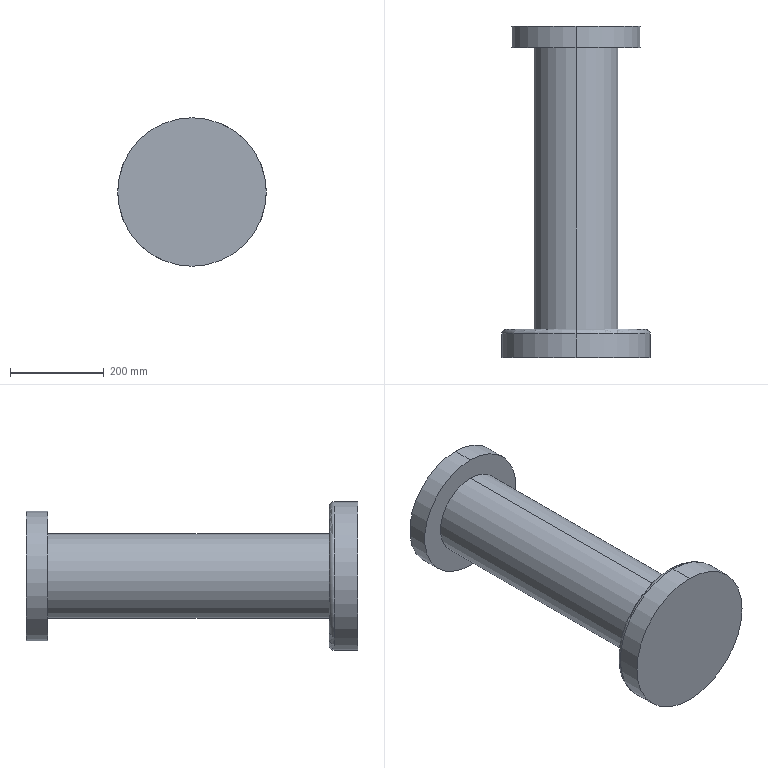Part | SolidWorks | features ICE 2, Extrusion 1, Fillet 1 | 1 solid | 12 faces | box 316.364 x 705 x 316.364 mm | volume 22636383 mm3 | cylinder 6 | plane 4 | torus 2 | commonest cylinder face diameters 180 x2 275 x2 316.364 x2
STEP:
#1=CARTESIAN_POINT('',(0.,-600.,148.182));
#2=VERTEX_POINT('',#1);
#3=CARTESIAN_POINT('',(0.,-600.,-148.182));
#4=VERTEX_POINT('',#3);
#5=CARTESIAN_POINT('',(0.,-600.,0.));
#6=DIRECTION('',(0.,1.,0.));
#7=DIRECTION('',(0.,0.,-1.));
#8=AXIS2_PLACEMENT_3D('',#5,#6,#7);
#9=CIRCLE('',#8,148.182);
#10=EDGE_CURVE('',#2,#4,#9,.T.);
#11=ORIENTED_EDGE('',*,*,#10,.F.);
#12=CARTESIAN_POINT('',(0.,-610.,158.182));
#13=VERTEX_POINT('',#12);
#14=CARTESIAN_POINT('',(0.,-610.,148.182));
#15=DIRECTION('',(1.,0.,0.));
#16=DIRECTION('',(0.,0.,-1.));
#17=AXIS2_PLACEMENT_3D('',#14,#15,#16);
#18=CIRCLE('',#17,10.);
#19=EDGE_CURVE('',#2,#13,#18,.T.);
#20=ORIENTED_EDGE('',*,*,#19,.T.);
#21=CARTESIAN_POINT('',(0.,-610.,-158.182));
#22=VERTEX_POINT('',#21);
#23=CARTESIAN_POINT('',(0.,-610.,0.));
#24=DIRECTION('',(0.,-1.,0.));
#25=DIRECTION('',(0.,0.,-1.));
#26=AXIS2_PLACEMENT_3D('',#23,#24,#25);
#27=CIRCLE('',#26,158.182);
#28=EDGE_CURVE('',#22,#13,#27,.T.);
#29=ORIENTED_EDGE('',*,*,#28,.F.);
#30=CARTESIAN_POINT('',(0.,-610.,-148.182));
#31=DIRECTION('',(-1.,0.,0.));
#32=DIRECTION('',(0.,0.,1.));
#33=AXIS2_PLACEMENT_3D('',#30,#31,#32);
#34=CIRCLE('',#33,10.);
#35=EDGE_CURVE('',#4,#22,#34,.T.);
#36=ORIENTED_EDGE('',*,*,#35,.F.);
#37=EDGE_LOOP('',(#11,#20,#29,#36));
#38=FACE_OUTER_BOUND('',#37,.T.);
#39=CARTESIAN_POINT('',(0.,-610.,0.));
#40=DIRECTION('',(0.,-1.,0.));
#41=DIRECTION('',(0.,0.,-1.));
#42=AXIS2_PLACEMENT_3D('',#39,#40,#41);
#43=TOROIDAL_SURFACE('',#42,148.182,10.);
#44=ADVANCED_FACE('',(#38),#43,.T.);
#45=CARTESIAN_POINT('',(0.,-660.,-158.182));
#46=VERTEX_POINT('',#45);
#47=CARTESIAN_POINT('',(0.,-660.,158.182));
#48=VERTEX_POINT('',#47);
#49=CARTESIAN_POINT('',(0.,-660.,0.));
#50=DIRECTION('',(0.,-1.,0.));
#51=DIRECTION('',(0.,0.,-1.));
#52=AXIS2_PLACEMENT_3D('',#49,#50,#51);
#53=CIRCLE('',#52,158.182);
#54=EDGE_CURVE('',#46,#48,#53,.T.);
#55=ORIENTED_EDGE('',*,*,#54,.F.);
#56=CARTESIAN_POINT('',(0.,-660.,-158.182));
#57=DIRECTION('',(0.,1.,0.));
#58=VECTOR('',#57,1000.);
#59=LINE('',#56,#58);
#60=EDGE_CURVE('',#46,#22,#59,.T.);
#61=ORIENTED_EDGE('',*,*,#60,.T.);
#62=ORIENTED_EDGE('',*,*,#28,.T.);
#63=CARTESIAN_POINT('',(0.,-660.,158.182));
#64=DIRECTION('',(0.,1.,0.));
#65=VECTOR('',#64,1000.);
#66=LINE('',#63,#65);
#67=EDGE_CURVE('',#48,#13,#66,.T.);
#68=ORIENTED_EDGE('',*,*,#67,.F.);
#69=EDGE_LOOP('',(#55,#61,#62,#68));
#70=FACE_OUTER_BOUND('',#69,.T.);
#71=CARTESIAN_POINT('',(0.,-660.,0.));
#72=DIRECTION('',(0.,1.,0.));
#73=DIRECTION('',(0.,0.,1.));
#74=AXIS2_PLACEMENT_3D('',#71,#72,#73);
#75=CYLINDRICAL_SURFACE('',#74,158.182);
#76=ADVANCED_FACE('',(#70),#75,.T.);
#77=CARTESIAN_POINT('',(0.,-600.,-90.));
#78=VERTEX_POINT('',#77);
#79=CARTESIAN_POINT('',(0.,-600.,90.));
#80=VERTEX_POINT('',#79);
#81=CARTESIAN_POINT('',(0.,-600.,0.));
#82=DIRECTION('',(0.,-1.,0.));
#83=DIRECTION('',(0.,0.,-1.));
#84=AXIS2_PLACEMENT_3D('',#81,#82,#83);
#85=CIRCLE('',#84,90.);
#86=EDGE_CURVE('',#78,#80,#85,.T.);
#87=ORIENTED_EDGE('',*,*,#86,.F.);
#88=CARTESIAN_POINT('',(0.,0.,-90.));
#89=VERTEX_POINT('',#88);
#90=CARTESIAN_POINT('',(0.,-600.,-90.));
#91=DIRECTION('',(0.,1.,0.));
#92=VECTOR('',#91,1000.);
#93=LINE('',#90,#92);
#94=EDGE_CURVE('',#78,#89,#93,.T.);
#95=ORIENTED_EDGE('',*,*,#94,.T.);
#96=CARTESIAN_POINT('',(0.,0.,90.));
#97=VERTEX_POINT('',#96);
#98=CARTESIAN_POINT('',(0.,0.,0.));
#99=DIRECTION('',(0.,-1.,0.));
#100=DIRECTION('',(0.,0.,1.));
#101=AXIS2_PLACEMENT_3D('',#98,#99,#100);
#102=CIRCLE('',#101,90.);
#103=EDGE_CURVE('',#89,#97,#102,.T.);
#104=ORIENTED_EDGE('',*,*,#103,.T.);
#105=CARTESIAN_POINT('',(0.,-600.,90.));
#106=DIRECTION('',(0.,1.,0.));
#107=VECTOR('',#106,1000.);
#108=LINE('',#105,#107);
#109=EDGE_CURVE('',#80,#97,#108,.T.);
#110=ORIENTED_EDGE('',*,*,#109,.F.);
#111=EDGE_LOOP('',(#87,#95,#104,#110));
#112=FACE_OUTER_BOUND('',#111,.T.);
#113=CARTESIAN_POINT('',(0.,-600.,0.));
#114=DIRECTION('',(0.,1.,0.));
#115=DIRECTION('',(0.,0.,1.));
#116=AXIS2_PLACEMENT_3D('',#113,#114,#115);
#117=CYLINDRICAL_SURFACE('',#116,90.);
#118=ADVANCED_FACE('',(#112),#117,.T.);
#119=CARTESIAN_POINT('',(0.,45.,137.5));
#120=VERTEX_POINT('',#119);
#121=CARTESIAN_POINT('',(0.,45.,-137.5));
#122=VERTEX_POINT('',#121);
#123=CARTESIAN_POINT('',(0.,45.,0.));
#124=DIRECTION('',(0.,1.,0.));
#125=DIRECTION('',(0.,0.,1.));
#126=AXIS2_PLACEMENT_3D('',#123,#124,#125);
#127=CIRCLE('',#126,137.5);
#128=EDGE_CURVE('',#120,#122,#127,.T.);
#129=ORIENTED_EDGE('',*,*,#128,.F.);
#130=CARTESIAN_POINT('',(0.,0.,137.5));
#131=VERTEX_POINT('',#130);
#132=CARTESIAN_POINT('',(0.,45.,137.5));
#133=DIRECTION('',(0.,-1.,0.));
#134=VECTOR('',#133,1000.);
#135=LINE('',#132,#134);
#136=EDGE_CURVE('',#120,#131,#135,.T.);
#137=ORIENTED_EDGE('',*,*,#136,.T.);
#138=CARTESIAN_POINT('',(0.,0.,-137.5));
#139=VERTEX_POINT('',#138);
#140=CARTESIAN_POINT('',(0.,0.,0.));
#141=DIRECTION('',(0.,1.,0.));
#142=DIRECTION('',(0.,0.,1.));
#143=AXIS2_PLACEMENT_3D('',#140,#141,#142);
#144=CIRCLE('',#143,137.5);
#145=EDGE_CURVE('',#131,#139,#144,.T.);
#146=ORIENTED_EDGE('',*,*,#145,.T.);
#147=CARTESIAN_POINT('',(0.,45.,-137.5));
#148=DIRECTION('',(0.,-1.,0.));
#149=VECTOR('',#148,1000.);
#150=LINE('',#147,#149);
#151=EDGE_CURVE('',#122,#139,#150,.T.);
#152=ORIENTED_EDGE('',*,*,#151,.F.);
#153=EDGE_LOOP('',(#129,#137,#146,#152));
#154=FACE_OUTER_BOUND('',#153,.T.);
#155=CARTESIAN_POINT('',(0.,45.,0.));
#156=DIRECTION('',(0.,-1.,0.));
#157=DIRECTION('',(0.,0.,-1.));
#158=AXIS2_PLACEMENT_3D('',#155,#156,#157);
#159=CYLINDRICAL_SURFACE('',#158,137.5);
#160=ADVANCED_FACE('',(#154),#159,.T.);
#161=ORIENTED_EDGE('',*,*,#136,.F.);
#162=CARTESIAN_POINT('',(0.,45.,0.));
#163=DIRECTION('',(0.,1.,0.));
#164=DIRECTION('',(0.,0.,1.));
#165=AXIS2_PLACEMENT_3D('',#162,#163,#164);
#166=CIRCLE('',#165,137.5);
#167=EDGE_CURVE('',#122,#120,#166,.T.);
#168=ORIENTED_EDGE('',*,*,#167,.F.);
#169=ORIENTED_EDGE('',*,*,#151,.T.);
#170=CARTESIAN_POINT('',(0.,0.,0.));
#171=DIRECTION('',(0.,1.,0.));
#172=DIRECTION('',(0.,0.,1.));
#173=AXIS2_PLACEMENT_3D('',#170,#171,#172);
#174=CIRCLE('',#173,137.5);
#175=EDGE_CURVE('',#139,#131,#174,.T.);
#176=ORIENTED_EDGE('',*,*,#175,.T.);
#177=EDGE_LOOP('',(#161,#168,#169,#176));
#178=FACE_OUTER_BOUND('',#177,.T.);
#179=CARTESIAN_POINT('',(0.,45.,0.));
#180=DIRECTION('',(0.,-1.,0.));
#181=DIRECTION('',(0.,0.,-1.));
#182=AXIS2_PLACEMENT_3D('',#179,#180,#181);
#183=CYLINDRICAL_SURFACE('',#182,137.5);
#184=ADVANCED_FACE('',(#178),#183,.T.);
#185=ORIENTED_EDGE('',*,*,#167,.T.);
#186=ORIENTED_EDGE('',*,*,#128,.T.);
#187=EDGE_LOOP('',(#185,#186));
#188=FACE_OUTER_BOUND('',#187,.T.);
#189=CARTESIAN_POINT('',(0.,45.,0.));
#190=DIRECTION('',(0.,1.,0.));
#191=DIRECTION('',(0.,0.,1.));
#192=AXIS2_PLACEMENT_3D('',#189,#190,#191);
#193=PLANE('',#192);
#194=ADVANCED_FACE('',(#188),#193,.T.);
#195=CARTESIAN_POINT('',(0.,0.,0.));
#196=DIRECTION('',(0.,-1.,0.));
#197=DIRECTION('',(0.,0.,1.));
#198=AXIS2_PLACEMENT_3D('',#195,#196,#197);
#199=CIRCLE('',#198,90.);
#200=EDGE_CURVE('',#97,#89,#199,.T.);
#201=ORIENTED_EDGE('',*,*,#200,.F.);
#202=ORIENTED_EDGE('',*,*,#103,.F.);
#203=EDGE_LOOP('',(#201,#202));
#204=FACE_BOUND('',#203,.T.);
#205=ORIENTED_EDGE('',*,*,#175,.F.);
#206=ORIENTED_EDGE('',*,*,#145,.F.);
#207=EDGE_LOOP('',(#205,#206));
#208=FACE_OUTER_BOUND('',#207,.T.);
#209=CARTESIAN_POINT('',(0.,0.,0.));
#210=DIRECTION('',(0.,1.,0.));
#211=DIRECTION('',(0.,0.,1.));
#212=AXIS2_PLACEMENT_3D('',#209,#210,#211);
#213=PLANE('',#212);
#214=ADVANCED_FACE('',(#204,#208),#213,.F.);
#215=ORIENTED_EDGE('',*,*,#94,.F.);
#216=CARTESIAN_POINT('',(0.,-600.,0.));
#217=DIRECTION('',(0.,-1.,0.));
#218=DIRECTION('',(0.,0.,-1.));
#219=AXIS2_PLACEMENT_3D('',#216,#217,#218);
#220=CIRCLE('',#219,90.);
#221=EDGE_CURVE('',#80,#78,#220,.T.);
#222=ORIENTED_EDGE('',*,*,#221,.F.);
#223=ORIENTED_EDGE('',*,*,#109,.T.);
#224=ORIENTED_EDGE('',*,*,#200,.T.);
#225=EDGE_LOOP('',(#215,#222,#223,#224));
#226=FACE_OUTER_BOUND('',#225,.T.);
#227=CARTESIAN_POINT('',(0.,-600.,0.));
#228=DIRECTION('',(0.,1.,0.));
#229=DIRECTION('',(0.,0.,1.));
#230=AXIS2_PLACEMENT_3D('',#227,#228,#229);
#231=CYLINDRICAL_SURFACE('',#230,90.);
#232=ADVANCED_FACE('',(#226),#231,.T.);
#233=ORIENTED_EDGE('',*,*,#60,.F.);
#234=CARTESIAN_POINT('',(0.,-660.,0.));
#235=DIRECTION('',(0.,-1.,0.));
#236=DIRECTION('',(0.,0.,-1.));
#237=AXIS2_PLACEMENT_3D('',#234,#235,#236);
#238=CIRCLE('',#237,158.182);
#239=EDGE_CURVE('',#48,#46,#238,.T.);
#240=ORIENTED_EDGE('',*,*,#239,.F.);
#241=ORIENTED_EDGE('',*,*,#67,.T.);
#242=CARTESIAN_POINT('',(0.,-610.,0.));
#243=DIRECTION('',(0.,-1.,0.));
#244=DIRECTION('',(0.,0.,-1.));
#245=AXIS2_PLACEMENT_3D('',#242,#243,#244);
#246=CIRCLE('',#245,158.182);
#247=EDGE_CURVE('',#13,#22,#246,.T.);
#248=ORIENTED_EDGE('',*,*,#247,.T.);
#249=EDGE_LOOP('',(#233,#240,#241,#248));
#250=FACE_OUTER_BOUND('',#249,.T.);
#251=CARTESIAN_POINT('',(0.,-660.,0.));
#252=DIRECTION('',(0.,1.,0.));
#253=DIRECTION('',(0.,0.,1.));
#254=AXIS2_PLACEMENT_3D('',#251,#252,#253);
#255=CYLINDRICAL_SURFACE('',#254,158.182);
#256=ADVANCED_FACE('',(#250),#255,.T.);
#257=ORIENTED_EDGE('',*,*,#239,.T.);
#258=ORIENTED_EDGE('',*,*,#54,.T.);
#259=EDGE_LOOP('',(#257,#258));
#260=FACE_OUTER_BOUND('',#259,.T.);
#261=CARTESIAN_POINT('',(0.,-660.,0.));
#262=DIRECTION('',(0.,-1.,0.));
#263=DIRECTION('',(0.,0.,-1.));
#264=AXIS2_PLACEMENT_3D('',#261,#262,#263);
#265=PLANE('',#264);
#266=ADVANCED_FACE('',(#260),#265,.T.);
#267=CARTESIAN_POINT('',(0.,-600.,0.));
#268=DIRECTION('',(0.,1.,0.));
#269=DIRECTION('',(0.,0.,-1.));
#270=AXIS2_PLACEMENT_3D('',#267,#268,#269);
#271=CIRCLE('',#270,148.182);
#272=EDGE_CURVE('',#4,#2,#271,.T.);
#273=ORIENTED_EDGE('',*,*,#272,.T.);
#274=ORIENTED_EDGE('',*,*,#10,.T.);
#275=EDGE_LOOP('',(#273,#274));
#276=FACE_OUTER_BOUND('',#275,.T.);
#277=ORIENTED_EDGE('',*,*,#221,.T.);
#278=ORIENTED_EDGE('',*,*,#86,.T.);
#279=EDGE_LOOP('',(#277,#278));
#280=FACE_BOUND('',#279,.T.);
#281=CARTESIAN_POINT('',(0.,-600.,0.));
#282=DIRECTION('',(0.,-1.,0.));
#283=DIRECTION('',(0.,0.,-1.));
#284=AXIS2_PLACEMENT_3D('',#281,#282,#283);
#285=PLANE('',#284);
#286=ADVANCED_FACE('',(#276,#280),#285,.F.);
#287=ORIENTED_EDGE('',*,*,#19,.F.);
#288=ORIENTED_EDGE('',*,*,#272,.F.);
#289=ORIENTED_EDGE('',*,*,#35,.T.);
#290=ORIENTED_EDGE('',*,*,#247,.F.);
#291=EDGE_LOOP('',(#287,#288,#289,#290));
#292=FACE_OUTER_BOUND('',#291,.T.);
#293=CARTESIAN_POINT('',(0.,-610.,0.));
#294=DIRECTION('',(0.,-1.,0.));
#295=DIRECTION('',(0.,0.,-1.));
#296=AXIS2_PLACEMENT_3D('',#293,#294,#295);
#297=TOROIDAL_SURFACE('',#296,148.182,10.);
#298=ADVANCED_FACE('',(#292),#297,.T.);
#299=CLOSED_SHELL('',(#44,#76,#118,#160,#184,#194,#214,#232,#256,#266,#286,#298));
#300=MANIFOLD_SOLID_BREP('',#299);
#301=CARTESIAN_POINT('',(0.,0.,0.));
#302=DIRECTION('',(0.,0.,1.));
#303=DIRECTION('',(1.,0.,0.));
#304=AXIS2_PLACEMENT_3D('',#301,#302,#303);
#305=(LENGTH_UNIT()NAMED_UNIT(*)SI_UNIT(.MILLI.,.METRE.));
#306=UNCERTAINTY_MEASURE_WITH_UNIT(LENGTH_MEASURE(0.00001),#305,'','');
#307=(NAMED_UNIT(*)PLANE_ANGLE_UNIT()SI_UNIT($,.RADIAN.));
#308=(NAMED_UNIT(*)SI_UNIT($,.STERADIAN.)SOLID_ANGLE_UNIT());
#309=(GEOMETRIC_REPRESENTATION_CONTEXT(3)GLOBAL_UNCERTAINTY_ASSIGNED_CONTEXT((#306))GLOBAL_UNIT_ASSIGNED_CONTEXT((#305,#307,#308))REPRESENTATION_CONTEXT('',''));
#310=ADVANCED_BREP_SHAPE_REPRESENTATION('',(#300,#304),#309);